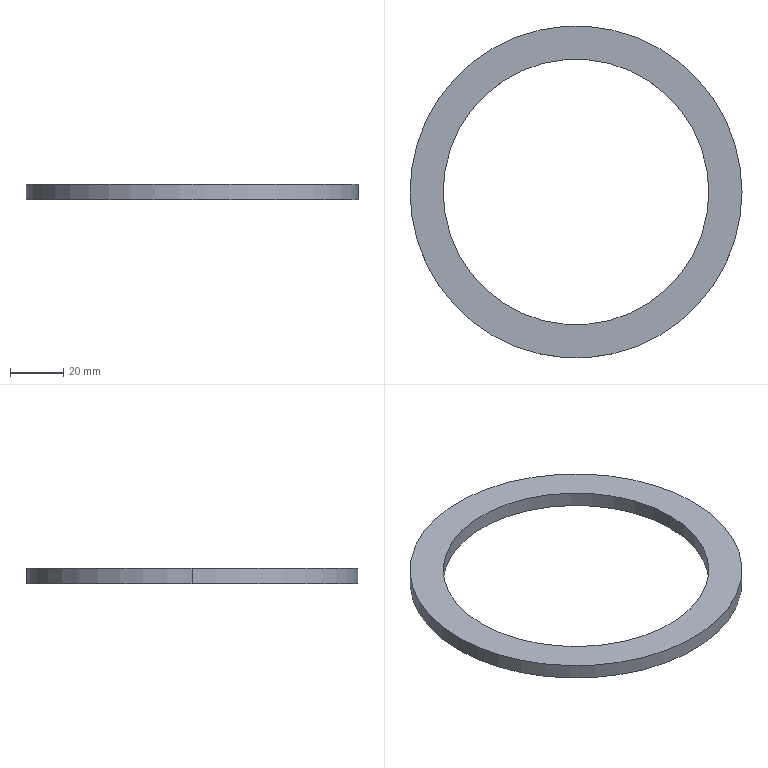Part | SolidWorks | features BaseBody 1 | 1 solid | 6 faces | box 125 x 125 x 5.7 mm | volume 25182 mm3 | cylinder 4 | plane 2 | commonest cylinder face diameters 100 x2 125 x2
STEP:
#1=CARTESIAN_POINT('',(-57.001,42.536,5.7));
#2=VERTEX_POINT('',#1);
#3=CARTESIAN_POINT('',(-157.001,42.536,5.7));
#4=VERTEX_POINT('',#3);
#5=CARTESIAN_POINT('',(-107.001,42.536,5.7));
#6=DIRECTION('',(0.,0.,-1.));
#7=DIRECTION('',(-1.,0.,0.));
#8=AXIS2_PLACEMENT_3D('',#5,#6,#7);
#9=CIRCLE('',#8,50.);
#10=EDGE_CURVE('',#2,#4,#9,.T.);
#11=ORIENTED_EDGE('',*,*,#10,.F.);
#12=CARTESIAN_POINT('',(-57.001,42.536,0.));
#13=VERTEX_POINT('',#12);
#14=CARTESIAN_POINT('',(-57.001,42.536,5.7));
#15=DIRECTION('',(0.,0.,-1.));
#16=VECTOR('',#15,1000.);
#17=LINE('',#14,#16);
#18=EDGE_CURVE('',#2,#13,#17,.T.);
#19=ORIENTED_EDGE('',*,*,#18,.T.);
#20=CARTESIAN_POINT('',(-157.001,42.536,0.));
#21=VERTEX_POINT('',#20);
#22=CARTESIAN_POINT('',(-107.001,42.536,0.));
#23=DIRECTION('',(0.,0.,1.));
#24=DIRECTION('',(-1.,0.,0.));
#25=AXIS2_PLACEMENT_3D('',#22,#23,#24);
#26=CIRCLE('',#25,50.);
#27=EDGE_CURVE('',#21,#13,#26,.T.);
#28=ORIENTED_EDGE('',*,*,#27,.F.);
#29=CARTESIAN_POINT('',(-157.001,42.536,5.7));
#30=DIRECTION('',(0.,0.,-1.));
#31=VECTOR('',#30,1000.);
#32=LINE('',#29,#31);
#33=EDGE_CURVE('',#4,#21,#32,.T.);
#34=ORIENTED_EDGE('',*,*,#33,.F.);
#35=EDGE_LOOP('',(#11,#19,#28,#34));
#36=FACE_OUTER_BOUND('',#35,.T.);
#37=CARTESIAN_POINT('',(-107.001,42.536,5.7));
#38=DIRECTION('',(0.,0.,-1.));
#39=DIRECTION('',(-1.,0.,0.));
#40=AXIS2_PLACEMENT_3D('',#37,#38,#39);
#41=CYLINDRICAL_SURFACE('',#40,50.);
#42=ADVANCED_FACE('',(#36),#41,.F.);
#43=CARTESIAN_POINT('',(-44.501,42.536,5.7));
#44=VERTEX_POINT('',#43);
#45=CARTESIAN_POINT('',(-169.501,42.536,5.7));
#46=VERTEX_POINT('',#45);
#47=CARTESIAN_POINT('',(-107.001,42.536,5.7));
#48=DIRECTION('',(0.,0.,1.));
#49=DIRECTION('',(-1.,0.,0.));
#50=AXIS2_PLACEMENT_3D('',#47,#48,#49);
#51=CIRCLE('',#50,62.5);
#52=EDGE_CURVE('',#44,#46,#51,.T.);
#53=ORIENTED_EDGE('',*,*,#52,.F.);
#54=CARTESIAN_POINT('',(-44.501,42.536,0.));
#55=VERTEX_POINT('',#54);
#56=CARTESIAN_POINT('',(-44.501,42.536,5.7));
#57=DIRECTION('',(0.,0.,-1.));
#58=VECTOR('',#57,1000.);
#59=LINE('',#56,#58);
#60=EDGE_CURVE('',#44,#55,#59,.T.);
#61=ORIENTED_EDGE('',*,*,#60,.T.);
#62=CARTESIAN_POINT('',(-169.501,42.536,0.));
#63=VERTEX_POINT('',#62);
#64=CARTESIAN_POINT('',(-107.001,42.536,0.));
#65=DIRECTION('',(0.,0.,1.));
#66=DIRECTION('',(-1.,0.,0.));
#67=AXIS2_PLACEMENT_3D('',#64,#65,#66);
#68=CIRCLE('',#67,62.5);
#69=EDGE_CURVE('',#55,#63,#68,.T.);
#70=ORIENTED_EDGE('',*,*,#69,.T.);
#71=CARTESIAN_POINT('',(-169.501,42.536,5.7));
#72=DIRECTION('',(0.,0.,-1.));
#73=VECTOR('',#72,1000.);
#74=LINE('',#71,#73);
#75=EDGE_CURVE('',#46,#63,#74,.T.);
#76=ORIENTED_EDGE('',*,*,#75,.F.);
#77=EDGE_LOOP('',(#53,#61,#70,#76));
#78=FACE_OUTER_BOUND('',#77,.T.);
#79=CARTESIAN_POINT('',(-107.001,42.536,5.7));
#80=DIRECTION('',(0.,0.,-1.));
#81=DIRECTION('',(-1.,0.,0.));
#82=AXIS2_PLACEMENT_3D('',#79,#80,#81);
#83=CYLINDRICAL_SURFACE('',#82,62.5);
#84=ADVANCED_FACE('',(#78),#83,.T.);
#85=CARTESIAN_POINT('',(-107.001,42.536,5.7));
#86=DIRECTION('',(0.,0.,-1.));
#87=DIRECTION('',(-1.,0.,0.));
#88=AXIS2_PLACEMENT_3D('',#85,#86,#87);
#89=CIRCLE('',#88,50.);
#90=EDGE_CURVE('',#4,#2,#89,.T.);
#91=ORIENTED_EDGE('',*,*,#90,.T.);
#92=ORIENTED_EDGE('',*,*,#10,.T.);
#93=EDGE_LOOP('',(#91,#92));
#94=FACE_BOUND('',#93,.T.);
#95=CARTESIAN_POINT('',(-107.001,42.536,5.7));
#96=DIRECTION('',(0.,0.,1.));
#97=DIRECTION('',(-1.,0.,0.));
#98=AXIS2_PLACEMENT_3D('',#95,#96,#97);
#99=CIRCLE('',#98,62.5);
#100=EDGE_CURVE('',#46,#44,#99,.T.);
#101=ORIENTED_EDGE('',*,*,#100,.T.);
#102=ORIENTED_EDGE('',*,*,#52,.T.);
#103=EDGE_LOOP('',(#101,#102));
#104=FACE_OUTER_BOUND('',#103,.T.);
#105=CARTESIAN_POINT('',(-107.001,42.536,5.7));
#106=DIRECTION('',(0.,0.,1.));
#107=DIRECTION('',(1.,0.,0.));
#108=AXIS2_PLACEMENT_3D('',#105,#106,#107);
#109=PLANE('',#108);
#110=ADVANCED_FACE('',(#94,#104),#109,.T.);
#111=ORIENTED_EDGE('',*,*,#18,.F.);
#112=ORIENTED_EDGE('',*,*,#90,.F.);
#113=ORIENTED_EDGE('',*,*,#33,.T.);
#114=CARTESIAN_POINT('',(-107.001,42.536,0.));
#115=DIRECTION('',(0.,0.,1.));
#116=DIRECTION('',(-1.,0.,0.));
#117=AXIS2_PLACEMENT_3D('',#114,#115,#116);
#118=CIRCLE('',#117,50.);
#119=EDGE_CURVE('',#13,#21,#118,.T.);
#120=ORIENTED_EDGE('',*,*,#119,.F.);
#121=EDGE_LOOP('',(#111,#112,#113,#120));
#122=FACE_OUTER_BOUND('',#121,.T.);
#123=CARTESIAN_POINT('',(-107.001,42.536,5.7));
#124=DIRECTION('',(0.,0.,-1.));
#125=DIRECTION('',(-1.,0.,0.));
#126=AXIS2_PLACEMENT_3D('',#123,#124,#125);
#127=CYLINDRICAL_SURFACE('',#126,50.);
#128=ADVANCED_FACE('',(#122),#127,.F.);
#129=ORIENTED_EDGE('',*,*,#60,.F.);
#130=ORIENTED_EDGE('',*,*,#100,.F.);
#131=ORIENTED_EDGE('',*,*,#75,.T.);
#132=CARTESIAN_POINT('',(-107.001,42.536,0.));
#133=DIRECTION('',(0.,0.,1.));
#134=DIRECTION('',(-1.,0.,0.));
#135=AXIS2_PLACEMENT_3D('',#132,#133,#134);
#136=CIRCLE('',#135,62.5);
#137=EDGE_CURVE('',#63,#55,#136,.T.);
#138=ORIENTED_EDGE('',*,*,#137,.T.);
#139=EDGE_LOOP('',(#129,#130,#131,#138));
#140=FACE_OUTER_BOUND('',#139,.T.);
#141=CARTESIAN_POINT('',(-107.001,42.536,5.7));
#142=DIRECTION('',(0.,0.,-1.));
#143=DIRECTION('',(-1.,0.,0.));
#144=AXIS2_PLACEMENT_3D('',#141,#142,#143);
#145=CYLINDRICAL_SURFACE('',#144,62.5);
#146=ADVANCED_FACE('',(#140),#145,.T.);
#147=ORIENTED_EDGE('',*,*,#27,.T.);
#148=ORIENTED_EDGE('',*,*,#119,.T.);
#149=EDGE_LOOP('',(#147,#148));
#150=FACE_BOUND('',#149,.T.);
#151=ORIENTED_EDGE('',*,*,#137,.F.);
#152=ORIENTED_EDGE('',*,*,#69,.F.);
#153=EDGE_LOOP('',(#151,#152));
#154=FACE_OUTER_BOUND('',#153,.T.);
#155=CARTESIAN_POINT('',(-107.001,42.536,0.));
#156=DIRECTION('',(0.,0.,1.));
#157=DIRECTION('',(1.,0.,0.));
#158=AXIS2_PLACEMENT_3D('',#155,#156,#157);
#159=PLANE('',#158);
#160=ADVANCED_FACE('',(#150,#154),#159,.F.);
#161=CLOSED_SHELL('',(#42,#84,#110,#128,#146,#160));
#162=MANIFOLD_SOLID_BREP('',#161);
#163=CARTESIAN_POINT('',(0.,0.,0.));
#164=DIRECTION('',(0.,0.,1.));
#165=DIRECTION('',(1.,0.,0.));
#166=AXIS2_PLACEMENT_3D('',#163,#164,#165);
#167=(LENGTH_UNIT()NAMED_UNIT(*)SI_UNIT(.MILLI.,.METRE.));
#168=UNCERTAINTY_MEASURE_WITH_UNIT(LENGTH_MEASURE(0.00001),#167,'','');
#169=(NAMED_UNIT(*)PLANE_ANGLE_UNIT()SI_UNIT($,.RADIAN.));
#170=(NAMED_UNIT(*)SI_UNIT($,.STERADIAN.)SOLID_ANGLE_UNIT());
#171=(GEOMETRIC_REPRESENTATION_CONTEXT(3)GLOBAL_UNCERTAINTY_ASSIGNED_CONTEXT((#168))GLOBAL_UNIT_ASSIGNED_CONTEXT((#167,#169,#170))REPRESENTATION_CONTEXT('',''));
#172=ADVANCED_BREP_SHAPE_REPRESENTATION('',(#162,#166),#171);